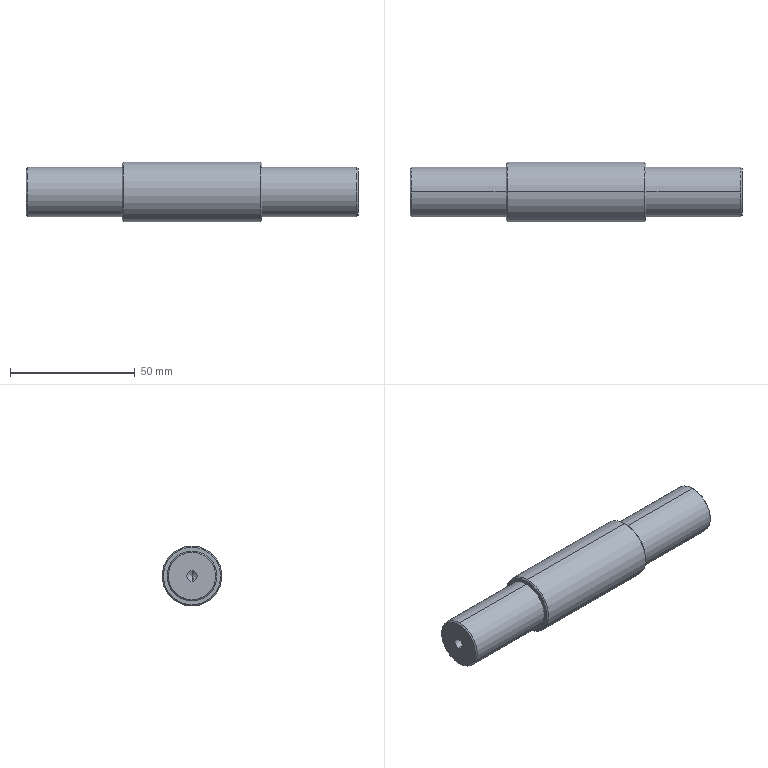Part | STEP file | 1 solid | 26 faces | box 133 x 24 x 24 mm | volume 49135 mm3 | cone 12 | cylinder 10 | plane 4 | commonest cylinder face diameters 4.2 x4 20 x4 24 x2